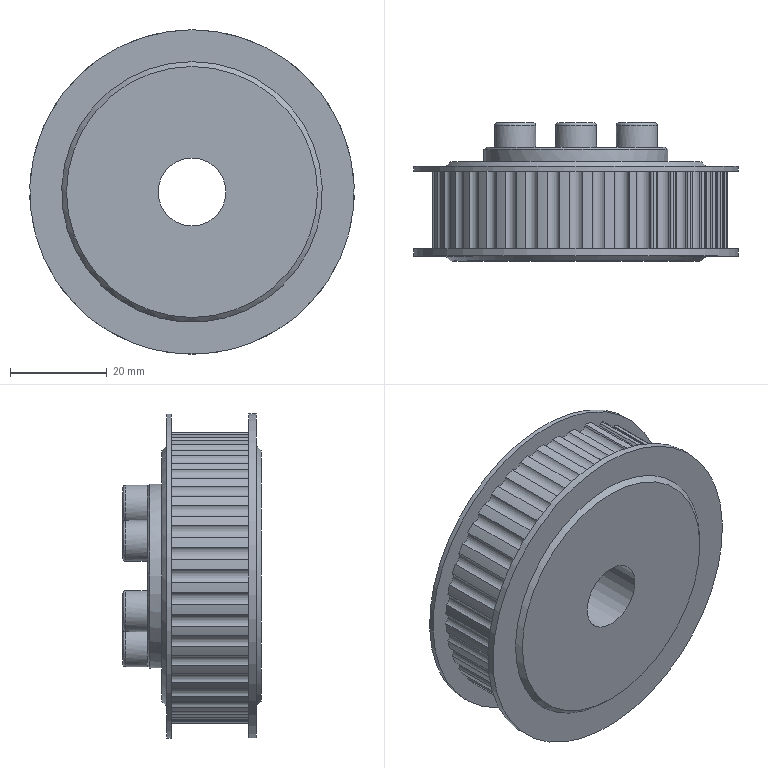Part | STEP file | 冲床-300配套压波_id318_x_t | 1 solid | 248 faces | box 67 x 28.5 x 67 mm | volume 58410 mm3 | cylinder 126 | plane 107 | cone 9 | torus 6 | commonest cylinder face diameters 3.12 x40 1 x33 59.52 x21 62.52 x16 4.2 x6 8.5 x6